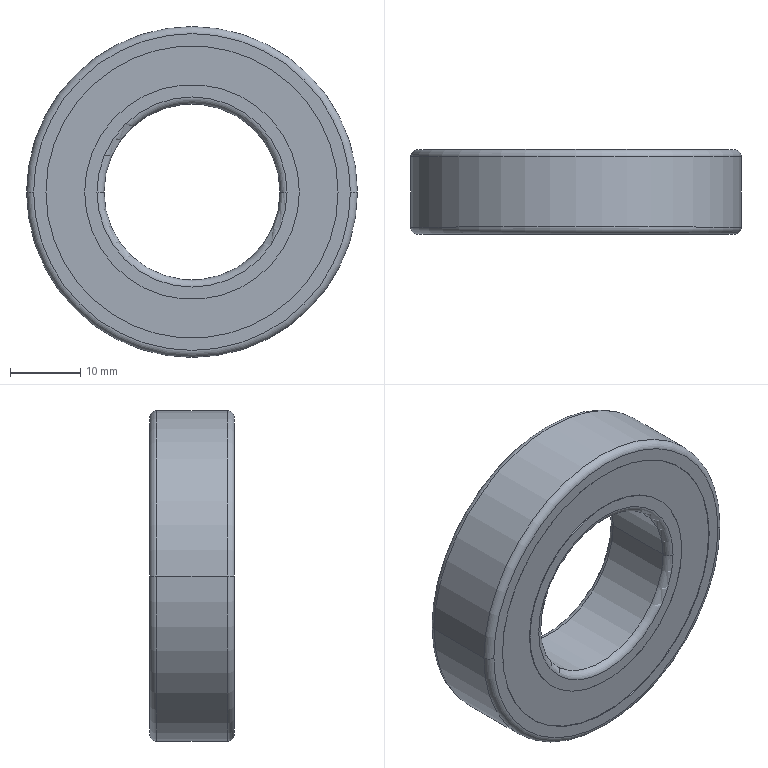Part | NX | 1 solid | 26 faces | box 47 x 12 x 47 mm | volume 14707 mm3 | cylinder 12 | torus 8 | plane 6 | commonest cylinder face diameters 30.5 x4 41.5 x4 25 x2 47 x2
STEP:
#1=CARTESIAN_POINT('',(-13.5,6.,0.));
#2=VERTEX_POINT('',#1);
#3=CARTESIAN_POINT('',(13.5,6.,0.));
#4=VERTEX_POINT('',#3);
#5=CARTESIAN_POINT('',(0.,6.,0.));
#6=DIRECTION('',(0.,1.,0.));
#7=DIRECTION('',(-1.,0.,0.));
#8=AXIS2_PLACEMENT_3D('',#5,#6,#7);
#9=CIRCLE('',#8,13.5);
#10=EDGE_CURVE('',#2,#4,#9,.T.);
#11=ORIENTED_EDGE('',*,*,#10,.T.);
#12=CARTESIAN_POINT('',(12.5,5.,0.));
#13=VERTEX_POINT('',#12);
#14=CARTESIAN_POINT('',(13.5,5.,0.));
#15=DIRECTION('',(0.,0.,1.));
#16=DIRECTION('',(1.,0.,0.));
#17=AXIS2_PLACEMENT_3D('',#14,#15,#16);
#18=CIRCLE('',#17,1.);
#19=EDGE_CURVE('',#4,#13,#18,.T.);
#20=ORIENTED_EDGE('',*,*,#19,.T.);
#21=CARTESIAN_POINT('',(-12.5,5.,0.));
#22=VERTEX_POINT('',#21);
#23=CARTESIAN_POINT('',(0.,5.,0.));
#24=DIRECTION('',(0.,-1.,0.));
#25=DIRECTION('',(-1.,0.,0.));
#26=AXIS2_PLACEMENT_3D('',#23,#24,#25);
#27=CIRCLE('',#26,12.5);
#28=EDGE_CURVE('',#13,#22,#27,.T.);
#29=ORIENTED_EDGE('',*,*,#28,.T.);
#30=CARTESIAN_POINT('',(-13.5,5.,0.));
#31=DIRECTION('',(0.,0.,-1.));
#32=DIRECTION('',(-1.,0.,0.));
#33=AXIS2_PLACEMENT_3D('',#30,#31,#32);
#34=CIRCLE('',#33,1.);
#35=EDGE_CURVE('',#2,#22,#34,.T.);
#36=ORIENTED_EDGE('',*,*,#35,.F.);
#37=EDGE_LOOP('',(#11,#20,#29,#36));
#38=FACE_BOUND('',#37,.T.);
#39=CARTESIAN_POINT('',(0.,5.,0.));
#40=DIRECTION('',(0.,-1.,0.));
#41=DIRECTION('',(-1.,0.,0.));
#42=AXIS2_PLACEMENT_3D('',#39,#40,#41);
#43=TOROIDAL_SURFACE('',#42,13.5,1.);
#44=ADVANCED_FACE('',(#38),#43,.T.);
#45=CARTESIAN_POINT('',(22.5,6.,0.));
#46=VERTEX_POINT('',#45);
#47=CARTESIAN_POINT('',(-22.5,6.,0.));
#48=VERTEX_POINT('',#47);
#49=CARTESIAN_POINT('',(0.,6.,0.));
#50=DIRECTION('',(0.,-1.,0.));
#51=DIRECTION('',(1.,0.,0.));
#52=AXIS2_PLACEMENT_3D('',#49,#50,#51);
#53=CIRCLE('',#52,22.5);
#54=EDGE_CURVE('',#46,#48,#53,.T.);
#55=ORIENTED_EDGE('',*,*,#54,.T.);
#56=CARTESIAN_POINT('',(-23.5,5.,0.));
#57=VERTEX_POINT('',#56);
#58=CARTESIAN_POINT('',(-22.5,5.,0.));
#59=DIRECTION('',(0.,0.,-1.));
#60=DIRECTION('',(-1.,0.,0.));
#61=AXIS2_PLACEMENT_3D('',#58,#59,#60);
#62=CIRCLE('',#61,1.);
#63=EDGE_CURVE('',#48,#57,#62,.F.);
#64=ORIENTED_EDGE('',*,*,#63,.T.);
#65=CARTESIAN_POINT('',(23.5,5.,0.));
#66=VERTEX_POINT('',#65);
#67=CARTESIAN_POINT('',(0.,5.,0.));
#68=DIRECTION('',(0.,-1.,0.));
#69=DIRECTION('',(-1.,0.,0.));
#70=AXIS2_PLACEMENT_3D('',#67,#68,#69);
#71=CIRCLE('',#70,23.5);
#72=EDGE_CURVE('',#66,#57,#71,.T.);
#73=ORIENTED_EDGE('',*,*,#72,.F.);
#74=CARTESIAN_POINT('',(22.5,5.,0.));
#75=DIRECTION('',(0.,0.,1.));
#76=DIRECTION('',(1.,0.,0.));
#77=AXIS2_PLACEMENT_3D('',#74,#75,#76);
#78=CIRCLE('',#77,1.);
#79=EDGE_CURVE('',#46,#66,#78,.F.);
#80=ORIENTED_EDGE('',*,*,#79,.F.);
#81=EDGE_LOOP('',(#55,#64,#73,#80));
#82=FACE_BOUND('',#81,.T.);
#83=CARTESIAN_POINT('',(0.,5.,0.));
#84=DIRECTION('',(0.,-1.,0.));
#85=DIRECTION('',(-1.,0.,0.));
#86=AXIS2_PLACEMENT_3D('',#83,#84,#85);
#87=TOROIDAL_SURFACE('',#86,22.5,1.);
#88=ADVANCED_FACE('',(#82),#87,.T.);
#89=CARTESIAN_POINT('',(0.,5.,0.));
#90=DIRECTION('',(0.,-1.,0.));
#91=DIRECTION('',(-1.,0.,0.));
#92=AXIS2_PLACEMENT_3D('',#89,#90,#91);
#93=CIRCLE('',#92,12.5);
#94=EDGE_CURVE('',#22,#13,#93,.T.);
#95=ORIENTED_EDGE('',*,*,#94,.F.);
#96=CARTESIAN_POINT('',(-12.5,-5.,0.));
#97=VERTEX_POINT('',#96);
#98=CARTESIAN_POINT('',(-12.5,6.6,0.));
#99=DIRECTION('',(0.,-1.,0.));
#100=VECTOR('',#99,1000.);
#101=LINE('',#98,#100);
#102=EDGE_CURVE('',#97,#22,#101,.F.);
#103=ORIENTED_EDGE('',*,*,#102,.F.);
#104=CARTESIAN_POINT('',(12.5,-5.,0.));
#105=VERTEX_POINT('',#104);
#106=CARTESIAN_POINT('',(0.,-5.,0.));
#107=DIRECTION('',(0.,-1.,0.));
#108=DIRECTION('',(-1.,0.,0.));
#109=AXIS2_PLACEMENT_3D('',#106,#107,#108);
#110=CIRCLE('',#109,12.5);
#111=EDGE_CURVE('',#97,#105,#110,.T.);
#112=ORIENTED_EDGE('',*,*,#111,.T.);
#113=CARTESIAN_POINT('',(12.5,6.6,0.));
#114=DIRECTION('',(0.,-1.,0.));
#115=VECTOR('',#114,1000.);
#116=LINE('',#113,#115);
#117=EDGE_CURVE('',#105,#13,#116,.F.);
#118=ORIENTED_EDGE('',*,*,#117,.T.);
#119=EDGE_LOOP('',(#95,#103,#112,#118));
#120=FACE_BOUND('',#119,.T.);
#121=CARTESIAN_POINT('',(0.,6.6,0.));
#122=DIRECTION('',(0.,-1.,0.));
#123=DIRECTION('',(-1.,0.,0.));
#124=AXIS2_PLACEMENT_3D('',#121,#122,#123);
#125=CYLINDRICAL_SURFACE('',#124,12.5);
#126=ADVANCED_FACE('',(#120),#125,.F.);
#127=CARTESIAN_POINT('',(-20.75,5.9,0.));
#128=VERTEX_POINT('',#127);
#129=CARTESIAN_POINT('',(20.75,5.9,0.));
#130=VERTEX_POINT('',#129);
#131=CARTESIAN_POINT('',(0.,5.9,0.));
#132=DIRECTION('',(0.,-1.,0.));
#133=DIRECTION('',(1.,0.,0.));
#134=AXIS2_PLACEMENT_3D('',#131,#132,#133);
#135=CIRCLE('',#134,20.75);
#136=EDGE_CURVE('',#128,#130,#135,.T.);
#137=ORIENTED_EDGE('',*,*,#136,.T.);
#138=CARTESIAN_POINT('',(20.75,6.,0.));
#139=VERTEX_POINT('',#138);
#140=CARTESIAN_POINT('',(20.75,6.6,0.));
#141=DIRECTION('',(0.,-1.,0.));
#142=VECTOR('',#141,1000.);
#143=LINE('',#140,#142);
#144=EDGE_CURVE('',#139,#130,#143,.T.);
#145=ORIENTED_EDGE('',*,*,#144,.F.);
#146=CARTESIAN_POINT('',(-20.75,6.,0.));
#147=VERTEX_POINT('',#146);
#148=CARTESIAN_POINT('',(0.,6.,0.));
#149=DIRECTION('',(0.,1.,0.));
#150=DIRECTION('',(1.,0.,0.));
#151=AXIS2_PLACEMENT_3D('',#148,#149,#150);
#152=CIRCLE('',#151,20.75);
#153=EDGE_CURVE('',#139,#147,#152,.T.);
#154=ORIENTED_EDGE('',*,*,#153,.T.);
#155=CARTESIAN_POINT('',(-20.75,6.6,0.));
#156=DIRECTION('',(0.,-1.,0.));
#157=VECTOR('',#156,1000.);
#158=LINE('',#155,#157);
#159=EDGE_CURVE('',#147,#128,#158,.T.);
#160=ORIENTED_EDGE('',*,*,#159,.T.);
#161=EDGE_LOOP('',(#137,#145,#154,#160));
#162=FACE_BOUND('',#161,.T.);
#163=CARTESIAN_POINT('',(0.,6.6,0.));
#164=DIRECTION('',(0.,-1.,0.));
#165=DIRECTION('',(-1.,0.,0.));
#166=AXIS2_PLACEMENT_3D('',#163,#164,#165);
#167=CYLINDRICAL_SURFACE('',#166,20.75);
#168=ADVANCED_FACE('',(#162),#167,.F.);
#169=ORIENTED_EDGE('',*,*,#111,.F.);
#170=CARTESIAN_POINT('',(-13.5,-6.,0.));
#171=VERTEX_POINT('',#170);
#172=CARTESIAN_POINT('',(-13.5,-5.,0.));
#173=DIRECTION('',(0.,0.,-1.));
#174=DIRECTION('',(-1.,0.,0.));
#175=AXIS2_PLACEMENT_3D('',#172,#173,#174);
#176=CIRCLE('',#175,1.);
#177=EDGE_CURVE('',#171,#97,#176,.F.);
#178=ORIENTED_EDGE('',*,*,#177,.F.);
#179=CARTESIAN_POINT('',(13.5,-6.,0.));
#180=VERTEX_POINT('',#179);
#181=CARTESIAN_POINT('',(0.,-6.,0.));
#182=DIRECTION('',(0.,-1.,0.));
#183=DIRECTION('',(1.,0.,0.));
#184=AXIS2_PLACEMENT_3D('',#181,#182,#183);
#185=CIRCLE('',#184,13.5);
#186=EDGE_CURVE('',#171,#180,#185,.T.);
#187=ORIENTED_EDGE('',*,*,#186,.T.);
#188=CARTESIAN_POINT('',(13.5,-5.,0.));
#189=DIRECTION('',(0.,0.,1.));
#190=DIRECTION('',(1.,0.,0.));
#191=AXIS2_PLACEMENT_3D('',#188,#189,#190);
#192=CIRCLE('',#191,1.);
#193=EDGE_CURVE('',#180,#105,#192,.F.);
#194=ORIENTED_EDGE('',*,*,#193,.T.);
#195=EDGE_LOOP('',(#169,#178,#187,#194));
#196=FACE_BOUND('',#195,.T.);
#197=CARTESIAN_POINT('',(0.,-5.,0.));
#198=DIRECTION('',(0.,-1.,0.));
#199=DIRECTION('',(-1.,0.,0.));
#200=AXIS2_PLACEMENT_3D('',#197,#198,#199);
#201=TOROIDAL_SURFACE('',#200,13.5,1.);
#202=ADVANCED_FACE('',(#196),#201,.T.);
#203=ORIENTED_EDGE('',*,*,#54,.F.);
#204=CARTESIAN_POINT('',(0.,6.,0.));
#205=DIRECTION('',(0.,-1.,0.));
#206=DIRECTION('',(1.,0.,0.));
#207=AXIS2_PLACEMENT_3D('',#204,#205,#206);
#208=CIRCLE('',#207,22.5);
#209=EDGE_CURVE('',#48,#46,#208,.T.);
#210=ORIENTED_EDGE('',*,*,#209,.F.);
#211=EDGE_LOOP('',(#203,#210));
#212=FACE_BOUND('',#211,.T.);
#213=CARTESIAN_POINT('',(0.,6.,0.));
#214=DIRECTION('',(0.,1.,0.));
#215=DIRECTION('',(1.,0.,0.));
#216=AXIS2_PLACEMENT_3D('',#213,#214,#215);
#217=CIRCLE('',#216,20.75);
#218=EDGE_CURVE('',#147,#139,#217,.T.);
#219=ORIENTED_EDGE('',*,*,#218,.F.);
#220=ORIENTED_EDGE('',*,*,#153,.F.);
#221=EDGE_LOOP('',(#219,#220));
#222=FACE_BOUND('',#221,.T.);
#223=CARTESIAN_POINT('',(0.,6.,0.));
#224=DIRECTION('',(0.,-1.,0.));
#225=DIRECTION('',(0.,0.,-1.));
#226=AXIS2_PLACEMENT_3D('',#223,#224,#225);
#227=PLANE('',#226);
#228=ADVANCED_FACE('',(#212,#222),#227,.F.);
#229=CARTESIAN_POINT('',(15.25,-6.,0.));
#230=VERTEX_POINT('',#229);
#231=CARTESIAN_POINT('',(-15.25,-6.,0.));
#232=VERTEX_POINT('',#231);
#233=CARTESIAN_POINT('',(0.,-6.,0.));
#234=DIRECTION('',(0.,1.,0.));
#235=DIRECTION('',(1.,0.,0.));
#236=AXIS2_PLACEMENT_3D('',#233,#234,#235);
#237=CIRCLE('',#236,15.25);
#238=EDGE_CURVE('',#230,#232,#237,.T.);
#239=ORIENTED_EDGE('',*,*,#238,.F.);
#240=CARTESIAN_POINT('',(0.,-6.,0.));
#241=DIRECTION('',(0.,1.,0.));
#242=DIRECTION('',(1.,0.,0.));
#243=AXIS2_PLACEMENT_3D('',#240,#241,#242);
#244=CIRCLE('',#243,15.25);
#245=EDGE_CURVE('',#232,#230,#244,.T.);
#246=ORIENTED_EDGE('',*,*,#245,.F.);
#247=EDGE_LOOP('',(#239,#246));
#248=FACE_BOUND('',#247,.T.);
#249=CARTESIAN_POINT('',(0.,-6.,0.));
#250=DIRECTION('',(0.,-1.,0.));
#251=DIRECTION('',(1.,0.,0.));
#252=AXIS2_PLACEMENT_3D('',#249,#250,#251);
#253=CIRCLE('',#252,13.5);
#254=EDGE_CURVE('',#180,#171,#253,.T.);
#255=ORIENTED_EDGE('',*,*,#254,.F.);
#256=ORIENTED_EDGE('',*,*,#186,.F.);
#257=EDGE_LOOP('',(#255,#256));
#258=FACE_BOUND('',#257,.T.);
#259=CARTESIAN_POINT('',(0.,-6.,0.));
#260=DIRECTION('',(0.,-1.,0.));
#261=DIRECTION('',(0.,0.,-1.));
#262=AXIS2_PLACEMENT_3D('',#259,#260,#261);
#263=PLANE('',#262);
#264=ADVANCED_FACE('',(#248,#258),#263,.T.);
#265=ORIENTED_EDGE('',*,*,#238,.T.);
#266=CARTESIAN_POINT('',(-15.25,-5.9,0.));
#267=VERTEX_POINT('',#266);
#268=CARTESIAN_POINT('',(-15.25,6.6,0.));
#269=DIRECTION('',(0.,-1.,0.));
#270=VECTOR('',#269,1000.);
#271=LINE('',#268,#270);
#272=EDGE_CURVE('',#232,#267,#271,.F.);
#273=ORIENTED_EDGE('',*,*,#272,.T.);
#274=CARTESIAN_POINT('',(15.25,-5.9,0.));
#275=VERTEX_POINT('',#274);
#276=CARTESIAN_POINT('',(0.,-5.9,0.));
#277=DIRECTION('',(0.,-1.,0.));
#278=DIRECTION('',(1.,0.,0.));
#279=AXIS2_PLACEMENT_3D('',#276,#277,#278);
#280=CIRCLE('',#279,15.25);
#281=EDGE_CURVE('',#267,#275,#280,.T.);
#282=ORIENTED_EDGE('',*,*,#281,.T.);
#283=CARTESIAN_POINT('',(15.25,6.6,0.));
#284=DIRECTION('',(0.,-1.,0.));
#285=VECTOR('',#284,1000.);
#286=LINE('',#283,#285);
#287=EDGE_CURVE('',#230,#275,#286,.F.);
#288=ORIENTED_EDGE('',*,*,#287,.F.);
#289=EDGE_LOOP('',(#265,#273,#282,#288));
#290=FACE_BOUND('',#289,.T.);
#291=CARTESIAN_POINT('',(0.,6.6,0.));
#292=DIRECTION('',(0.,-1.,0.));
#293=DIRECTION('',(-1.,0.,0.));
#294=AXIS2_PLACEMENT_3D('',#291,#292,#293);
#295=CYLINDRICAL_SURFACE('',#294,15.25);
#296=ADVANCED_FACE('',(#290),#295,.T.);
#297=CARTESIAN_POINT('',(15.25,6.,0.));
#298=VERTEX_POINT('',#297);
#299=CARTESIAN_POINT('',(-15.25,6.,0.));
#300=VERTEX_POINT('',#299);
#301=CARTESIAN_POINT('',(0.,6.,0.));
#302=DIRECTION('',(0.,-1.,0.));
#303=DIRECTION('',(1.,0.,0.));
#304=AXIS2_PLACEMENT_3D('',#301,#302,#303);
#305=CIRCLE('',#304,15.25);
#306=EDGE_CURVE('',#298,#300,#305,.T.);
#307=ORIENTED_EDGE('',*,*,#306,.F.);
#308=CARTESIAN_POINT('',(0.,6.,0.));
#309=DIRECTION('',(0.,-1.,0.));
#310=DIRECTION('',(1.,0.,0.));
#311=AXIS2_PLACEMENT_3D('',#308,#309,#310);
#312=CIRCLE('',#311,15.25);
#313=EDGE_CURVE('',#300,#298,#312,.T.);
#314=ORIENTED_EDGE('',*,*,#313,.F.);
#315=EDGE_LOOP('',(#307,#314));
#316=FACE_BOUND('',#315,.T.);
#317=ORIENTED_EDGE('',*,*,#10,.F.);
#318=CARTESIAN_POINT('',(0.,6.,0.));
#319=DIRECTION('',(0.,1.,0.));
#320=DIRECTION('',(-1.,0.,0.));
#321=AXIS2_PLACEMENT_3D('',#318,#319,#320);
#322=CIRCLE('',#321,13.5);
#323=EDGE_CURVE('',#4,#2,#322,.T.);
#324=ORIENTED_EDGE('',*,*,#323,.F.);
#325=EDGE_LOOP('',(#317,#324));
#326=FACE_BOUND('',#325,.T.);
#327=CARTESIAN_POINT('',(0.,6.,0.));
#328=DIRECTION('',(0.,-1.,0.));
#329=DIRECTION('',(0.,0.,-1.));
#330=AXIS2_PLACEMENT_3D('',#327,#328,#329);
#331=PLANE('',#330);
#332=ADVANCED_FACE('',(#316,#326),#331,.F.);
#333=CARTESIAN_POINT('',(20.75,-5.9,0.));
#334=VERTEX_POINT('',#333);
#335=CARTESIAN_POINT('',(-20.75,-5.9,0.));
#336=VERTEX_POINT('',#335);
#337=CARTESIAN_POINT('',(0.,-5.9,0.));
#338=DIRECTION('',(0.,1.,0.));
#339=DIRECTION('',(1.,0.,0.));
#340=AXIS2_PLACEMENT_3D('',#337,#338,#339);
#341=CIRCLE('',#340,20.75);
#342=EDGE_CURVE('',#334,#336,#341,.T.);
#343=ORIENTED_EDGE('',*,*,#342,.F.);
#344=CARTESIAN_POINT('',(0.,-5.9,0.));
#345=DIRECTION('',(0.,1.,0.));
#346=DIRECTION('',(1.,0.,0.));
#347=AXIS2_PLACEMENT_3D('',#344,#345,#346);
#348=CIRCLE('',#347,20.75);
#349=EDGE_CURVE('',#336,#334,#348,.T.);
#350=ORIENTED_EDGE('',*,*,#349,.F.);
#351=EDGE_LOOP('',(#343,#350));
#352=FACE_BOUND('',#351,.T.);
#353=CARTESIAN_POINT('',(0.,-5.9,0.));
#354=DIRECTION('',(0.,-1.,0.));
#355=DIRECTION('',(1.,0.,0.));
#356=AXIS2_PLACEMENT_3D('',#353,#354,#355);
#357=CIRCLE('',#356,15.25);
#358=EDGE_CURVE('',#275,#267,#357,.T.);
#359=ORIENTED_EDGE('',*,*,#358,.F.);
#360=ORIENTED_EDGE('',*,*,#281,.F.);
#361=EDGE_LOOP('',(#359,#360));
#362=FACE_BOUND('',#361,.T.);
#363=CARTESIAN_POINT('',(0.,-5.9,0.));
#364=DIRECTION('',(0.,-1.,0.));
#365=DIRECTION('',(0.,0.,-1.));
#366=AXIS2_PLACEMENT_3D('',#363,#364,#365);
#367=PLANE('',#366);
#368=ADVANCED_FACE('',(#352,#362),#367,.T.);
#369=ORIENTED_EDGE('',*,*,#342,.T.);
#370=CARTESIAN_POINT('',(-20.75,-6.,0.));
#371=VERTEX_POINT('',#370);
#372=CARTESIAN_POINT('',(-20.75,6.6,0.));
#373=DIRECTION('',(0.,-1.,0.));
#374=VECTOR('',#373,1000.);
#375=LINE('',#372,#374);
#376=EDGE_CURVE('',#371,#336,#375,.F.);
#377=ORIENTED_EDGE('',*,*,#376,.F.);
#378=CARTESIAN_POINT('',(20.75,-6.,0.));
#379=VERTEX_POINT('',#378);
#380=CARTESIAN_POINT('',(0.,-6.,0.));
#381=DIRECTION('',(0.,-1.,0.));
#382=DIRECTION('',(1.,0.,0.));
#383=AXIS2_PLACEMENT_3D('',#380,#381,#382);
#384=CIRCLE('',#383,20.75);
#385=EDGE_CURVE('',#371,#379,#384,.T.);
#386=ORIENTED_EDGE('',*,*,#385,.T.);
#387=CARTESIAN_POINT('',(20.75,6.6,0.));
#388=DIRECTION('',(0.,-1.,0.));
#389=VECTOR('',#388,1000.);
#390=LINE('',#387,#389);
#391=EDGE_CURVE('',#379,#334,#390,.F.);
#392=ORIENTED_EDGE('',*,*,#391,.T.);
#393=EDGE_LOOP('',(#369,#377,#386,#392));
#394=FACE_BOUND('',#393,.T.);
#395=CARTESIAN_POINT('',(0.,6.6,0.));
#396=DIRECTION('',(0.,-1.,0.));
#397=DIRECTION('',(-1.,0.,0.));
#398=AXIS2_PLACEMENT_3D('',#395,#396,#397);
#399=CYLINDRICAL_SURFACE('',#398,20.75);
#400=ADVANCED_FACE('',(#394),#399,.F.);
#401=CARTESIAN_POINT('',(15.25,5.9,0.));
#402=VERTEX_POINT('',#401);
#403=CARTESIAN_POINT('',(-15.25,5.9,0.));
#404=VERTEX_POINT('',#403);
#405=CARTESIAN_POINT('',(0.,5.9,0.));
#406=DIRECTION('',(0.,1.,0.));
#407=DIRECTION('',(1.,0.,0.));
#408=AXIS2_PLACEMENT_3D('',#405,#406,#407);
#409=CIRCLE('',#408,15.25);
#410=EDGE_CURVE('',#402,#404,#409,.T.);
#411=ORIENTED_EDGE('',*,*,#410,.T.);
#412=CARTESIAN_POINT('',(-15.25,6.6,0.));
#413=DIRECTION('',(0.,-1.,0.));
#414=VECTOR('',#413,1000.);
#415=LINE('',#412,#414);
#416=EDGE_CURVE('',#404,#300,#415,.F.);
#417=ORIENTED_EDGE('',*,*,#416,.T.);
#418=ORIENTED_EDGE('',*,*,#313,.T.);
#419=CARTESIAN_POINT('',(15.25,6.6,0.));
#420=DIRECTION('',(0.,-1.,0.));
#421=VECTOR('',#420,1000.);
#422=LINE('',#419,#421);
#423=EDGE_CURVE('',#402,#298,#422,.F.);
#424=ORIENTED_EDGE('',*,*,#423,.F.);
#425=EDGE_LOOP('',(#411,#417,#418,#424));
#426=FACE_BOUND('',#425,.T.);
#427=CARTESIAN_POINT('',(0.,6.6,0.));
#428=DIRECTION('',(0.,-1.,0.));
#429=DIRECTION('',(-1.,0.,0.));
#430=AXIS2_PLACEMENT_3D('',#427,#428,#429);
#431=CYLINDRICAL_SURFACE('',#430,15.25);
#432=ADVANCED_FACE('',(#426),#431,.T.);
#433=CARTESIAN_POINT('',(22.5,-6.,0.));
#434=VERTEX_POINT('',#433);
#435=CARTESIAN_POINT('',(-22.5,-6.,0.));
#436=VERTEX_POINT('',#435);
#437=CARTESIAN_POINT('',(0.,-6.,0.));
#438=DIRECTION('',(0.,1.,0.));
#439=DIRECTION('',(1.,0.,0.));
#440=AXIS2_PLACEMENT_3D('',#437,#438,#439);
#441=CIRCLE('',#440,22.5);
#442=EDGE_CURVE('',#434,#436,#441,.T.);
#443=ORIENTED_EDGE('',*,*,#442,.F.);
#444=CARTESIAN_POINT('',(0.,-6.,0.));
#445=DIRECTION('',(0.,1.,0.));
#446=DIRECTION('',(1.,0.,0.));
#447=AXIS2_PLACEMENT_3D('',#444,#445,#446);
#448=CIRCLE('',#447,22.5);
#449=EDGE_CURVE('',#436,#434,#448,.T.);
#450=ORIENTED_EDGE('',*,*,#449,.F.);
#451=EDGE_LOOP('',(#443,#450));
#452=FACE_BOUND('',#451,.T.);
#453=ORIENTED_EDGE('',*,*,#385,.F.);
#454=CARTESIAN_POINT('',(0.,-6.,0.));
#455=DIRECTION('',(0.,-1.,0.));
#456=DIRECTION('',(1.,0.,0.));
#457=AXIS2_PLACEMENT_3D('',#454,#455,#456);
#458=CIRCLE('',#457,20.75);
#459=EDGE_CURVE('',#379,#371,#458,.T.);
#460=ORIENTED_EDGE('',*,*,#459,.F.);
#461=EDGE_LOOP('',(#453,#460));
#462=FACE_BOUND('',#461,.T.);
#463=CARTESIAN_POINT('',(0.,-6.,0.));
#464=DIRECTION('',(0.,-1.,0.));
#465=DIRECTION('',(0.,0.,-1.));
#466=AXIS2_PLACEMENT_3D('',#463,#464,#465);
#467=PLANE('',#466);
#468=ADVANCED_FACE('',(#452,#462),#467,.T.);
#469=ORIENTED_EDGE('',*,*,#442,.T.);
#470=CARTESIAN_POINT('',(-23.5,-5.,0.));
#471=VERTEX_POINT('',#470);
#472=CARTESIAN_POINT('',(-22.5,-5.,0.));
#473=DIRECTION('',(0.,0.,-1.));
#474=DIRECTION('',(-1.,0.,0.));
#475=AXIS2_PLACEMENT_3D('',#472,#473,#474);
#476=CIRCLE('',#475,1.);
#477=EDGE_CURVE('',#471,#436,#476,.F.);
#478=ORIENTED_EDGE('',*,*,#477,.F.);
#479=CARTESIAN_POINT('',(23.5,-5.,0.));
#480=VERTEX_POINT('',#479);
#481=CARTESIAN_POINT('',(0.,-5.,0.));
#482=DIRECTION('',(0.,-1.,0.));
#483=DIRECTION('',(-1.,0.,0.));
#484=AXIS2_PLACEMENT_3D('',#481,#482,#483);
#485=CIRCLE('',#484,23.5);
#486=EDGE_CURVE('',#471,#480,#485,.T.);
#487=ORIENTED_EDGE('',*,*,#486,.T.);
#488=CARTESIAN_POINT('',(22.5,-5.,0.));
#489=DIRECTION('',(0.,0.,1.));
#490=DIRECTION('',(1.,0.,0.));
#491=AXIS2_PLACEMENT_3D('',#488,#489,#490);
#492=CIRCLE('',#491,1.);
#493=EDGE_CURVE('',#480,#434,#492,.F.);
#494=ORIENTED_EDGE('',*,*,#493,.T.);
#495=EDGE_LOOP('',(#469,#478,#487,#494));
#496=FACE_BOUND('',#495,.T.);
#497=CARTESIAN_POINT('',(0.,-5.,0.));
#498=DIRECTION('',(0.,-1.,0.));
#499=DIRECTION('',(-1.,0.,0.));
#500=AXIS2_PLACEMENT_3D('',#497,#498,#499);
#501=TOROIDAL_SURFACE('',#500,22.5,1.);
#502=ADVANCED_FACE('',(#496),#501,.T.);
#503=ORIENTED_EDGE('',*,*,#136,.F.);
#504=CARTESIAN_POINT('',(0.,5.9,0.));
#505=DIRECTION('',(0.,-1.,0.));
#506=DIRECTION('',(1.,0.,0.));
#507=AXIS2_PLACEMENT_3D('',#504,#505,#506);
#508=CIRCLE('',#507,20.75);
#509=EDGE_CURVE('',#130,#128,#508,.T.);
#510=ORIENTED_EDGE('',*,*,#509,.F.);
#511=EDGE_LOOP('',(#503,#510));
#512=FACE_BOUND('',#511,.T.);
#513=ORIENTED_EDGE('',*,*,#410,.F.);
#514=CARTESIAN_POINT('',(0.,5.9,0.));
#515=DIRECTION('',(0.,1.,0.));
#516=DIRECTION('',(1.,0.,0.));
#517=AXIS2_PLACEMENT_3D('',#514,#515,#516);
#518=CIRCLE('',#517,15.25);
#519=EDGE_CURVE('',#404,#402,#518,.T.);
#520=ORIENTED_EDGE('',*,*,#519,.F.);
#521=EDGE_LOOP('',(#513,#520));
#522=FACE_BOUND('',#521,.T.);
#523=CARTESIAN_POINT('',(0.,5.9,0.));
#524=DIRECTION('',(0.,-1.,0.));
#525=DIRECTION('',(0.,0.,-1.));
#526=AXIS2_PLACEMENT_3D('',#523,#524,#525);
#527=PLANE('',#526);
#528=ADVANCED_FACE('',(#512,#522),#527,.F.);
#529=CARTESIAN_POINT('',(0.,-5.,0.));
#530=DIRECTION('',(0.,-1.,0.));
#531=DIRECTION('',(-1.,0.,0.));
#532=AXIS2_PLACEMENT_3D('',#529,#530,#531);
#533=CIRCLE('',#532,23.5);
#534=EDGE_CURVE('',#480,#471,#533,.T.);
#535=ORIENTED_EDGE('',*,*,#534,.F.);
#536=CARTESIAN_POINT('',(23.5,6.6,0.));
#537=DIRECTION('',(0.,-1.,0.));
#538=VECTOR('',#537,1000.);
#539=LINE('',#536,#538);
#540=EDGE_CURVE('',#480,#66,#539,.F.);
#541=ORIENTED_EDGE('',*,*,#540,.T.);
#542=ORIENTED_EDGE('',*,*,#72,.T.);
#543=CARTESIAN_POINT('',(-23.5,6.6,0.));
#544=DIRECTION('',(0.,-1.,0.));
#545=VECTOR('',#544,1000.);
#546=LINE('',#543,#545);
#547=EDGE_CURVE('',#471,#57,#546,.F.);
#548=ORIENTED_EDGE('',*,*,#547,.F.);
#549=EDGE_LOOP('',(#535,#541,#542,#548));
#550=FACE_BOUND('',#549,.T.);
#551=CARTESIAN_POINT('',(0.,6.6,0.));
#552=DIRECTION('',(0.,-1.,0.));
#553=DIRECTION('',(-1.,0.,0.));
#554=AXIS2_PLACEMENT_3D('',#551,#552,#553);
#555=CYLINDRICAL_SURFACE('',#554,23.5);
#556=ADVANCED_FACE('',(#550),#555,.T.);
#557=ORIENTED_EDGE('',*,*,#306,.T.);
#558=ORIENTED_EDGE('',*,*,#416,.F.);
#559=ORIENTED_EDGE('',*,*,#519,.T.);
#560=ORIENTED_EDGE('',*,*,#423,.T.);
#561=EDGE_LOOP('',(#557,#558,#559,#560));
#562=FACE_BOUND('',#561,.T.);
#563=CARTESIAN_POINT('',(0.,6.6,0.));
#564=DIRECTION('',(0.,-1.,0.));
#565=DIRECTION('',(-1.,0.,0.));
#566=AXIS2_PLACEMENT_3D('',#563,#564,#565);
#567=CYLINDRICAL_SURFACE('',#566,15.25);
#568=ADVANCED_FACE('',(#562),#567,.T.);
#569=ORIENTED_EDGE('',*,*,#102,.T.);
#570=ORIENTED_EDGE('',*,*,#28,.F.);
#571=ORIENTED_EDGE('',*,*,#117,.F.);
#572=CARTESIAN_POINT('',(0.,-5.,0.));
#573=DIRECTION('',(0.,-1.,0.));
#574=DIRECTION('',(-1.,0.,0.));
#575=AXIS2_PLACEMENT_3D('',#572,#573,#574);
#576=CIRCLE('',#575,12.5);
#577=EDGE_CURVE('',#105,#97,#576,.T.);
#578=ORIENTED_EDGE('',*,*,#577,.T.);
#579=EDGE_LOOP('',(#569,#570,#571,#578));
#580=FACE_BOUND('',#579,.T.);
#581=CARTESIAN_POINT('',(0.,6.6,0.));
#582=DIRECTION('',(0.,-1.,0.));
#583=DIRECTION('',(-1.,0.,0.));
#584=AXIS2_PLACEMENT_3D('',#581,#582,#583);
#585=CYLINDRICAL_SURFACE('',#584,12.5);
#586=ADVANCED_FACE('',(#580),#585,.F.);
#587=ORIENTED_EDGE('',*,*,#358,.T.);
#588=ORIENTED_EDGE('',*,*,#272,.F.);
#589=ORIENTED_EDGE('',*,*,#245,.T.);
#590=ORIENTED_EDGE('',*,*,#287,.T.);
#591=EDGE_LOOP('',(#587,#588,#589,#590));
#592=FACE_BOUND('',#591,.T.);
#593=CARTESIAN_POINT('',(0.,6.6,0.));
#594=DIRECTION('',(0.,-1.,0.));
#595=DIRECTION('',(-1.,0.,0.));
#596=AXIS2_PLACEMENT_3D('',#593,#594,#595);
#597=CYLINDRICAL_SURFACE('',#596,15.25);
#598=ADVANCED_FACE('',(#592),#597,.T.);
#599=ORIENTED_EDGE('',*,*,#376,.T.);
#600=ORIENTED_EDGE('',*,*,#349,.T.);
#601=ORIENTED_EDGE('',*,*,#391,.F.);
#602=ORIENTED_EDGE('',*,*,#459,.T.);
#603=EDGE_LOOP('',(#599,#600,#601,#602));
#604=FACE_BOUND('',#603,.T.);
#605=CARTESIAN_POINT('',(0.,6.6,0.));
#606=DIRECTION('',(0.,-1.,0.));
#607=DIRECTION('',(-1.,0.,0.));
#608=AXIS2_PLACEMENT_3D('',#605,#606,#607);
#609=CYLINDRICAL_SURFACE('',#608,20.75);
#610=ADVANCED_FACE('',(#604),#609,.F.);
#611=ORIENTED_EDGE('',*,*,#547,.T.);
#612=CARTESIAN_POINT('',(0.,5.,0.));
#613=DIRECTION('',(0.,-1.,0.));
#614=DIRECTION('',(-1.,0.,0.));
#615=AXIS2_PLACEMENT_3D('',#612,#613,#614);
#616=CIRCLE('',#615,23.5);
#617=EDGE_CURVE('',#57,#66,#616,.T.);
#618=ORIENTED_EDGE('',*,*,#617,.T.);
#619=ORIENTED_EDGE('',*,*,#540,.F.);
#620=ORIENTED_EDGE('',*,*,#486,.F.);
#621=EDGE_LOOP('',(#611,#618,#619,#620));
#622=FACE_BOUND('',#621,.T.);
#623=CARTESIAN_POINT('',(0.,6.6,0.));
#624=DIRECTION('',(0.,-1.,0.));
#625=DIRECTION('',(-1.,0.,0.));
#626=AXIS2_PLACEMENT_3D('',#623,#624,#625);
#627=CYLINDRICAL_SURFACE('',#626,23.5);
#628=ADVANCED_FACE('',(#622),#627,.T.);
#629=ORIENTED_EDGE('',*,*,#218,.T.);
#630=ORIENTED_EDGE('',*,*,#144,.T.);
#631=ORIENTED_EDGE('',*,*,#509,.T.);
#632=ORIENTED_EDGE('',*,*,#159,.F.);
#633=EDGE_LOOP('',(#629,#630,#631,#632));
#634=FACE_BOUND('',#633,.T.);
#635=CARTESIAN_POINT('',(0.,6.6,0.));
#636=DIRECTION('',(0.,-1.,0.));
#637=DIRECTION('',(-1.,0.,0.));
#638=AXIS2_PLACEMENT_3D('',#635,#636,#637);
#639=CYLINDRICAL_SURFACE('',#638,20.75);
#640=ADVANCED_FACE('',(#634),#639,.F.);
#641=ORIENTED_EDGE('',*,*,#254,.T.);
#642=ORIENTED_EDGE('',*,*,#177,.T.);
#643=ORIENTED_EDGE('',*,*,#577,.F.);
#644=ORIENTED_EDGE('',*,*,#193,.F.);
#645=EDGE_LOOP('',(#641,#642,#643,#644));
#646=FACE_BOUND('',#645,.T.);
#647=CARTESIAN_POINT('',(0.,-5.,0.));
#648=DIRECTION('',(0.,-1.,0.));
#649=DIRECTION('',(-1.,0.,0.));
#650=AXIS2_PLACEMENT_3D('',#647,#648,#649);
#651=TOROIDAL_SURFACE('',#650,13.5,1.);
#652=ADVANCED_FACE('',(#646),#651,.T.);
#653=ORIENTED_EDGE('',*,*,#534,.T.);
#654=ORIENTED_EDGE('',*,*,#477,.T.);
#655=ORIENTED_EDGE('',*,*,#449,.T.);
#656=ORIENTED_EDGE('',*,*,#493,.F.);
#657=EDGE_LOOP('',(#653,#654,#655,#656));
#658=FACE_BOUND('',#657,.T.);
#659=CARTESIAN_POINT('',(0.,-5.,0.));
#660=DIRECTION('',(0.,-1.,0.));
#661=DIRECTION('',(-1.,0.,0.));
#662=AXIS2_PLACEMENT_3D('',#659,#660,#661);
#663=TOROIDAL_SURFACE('',#662,22.5,1.);
#664=ADVANCED_FACE('',(#658),#663,.T.);
#665=ORIENTED_EDGE('',*,*,#63,.F.);
#666=ORIENTED_EDGE('',*,*,#209,.T.);
#667=ORIENTED_EDGE('',*,*,#79,.T.);
#668=ORIENTED_EDGE('',*,*,#617,.F.);
#669=EDGE_LOOP('',(#665,#666,#667,#668));
#670=FACE_BOUND('',#669,.T.);
#671=CARTESIAN_POINT('',(0.,5.,0.));
#672=DIRECTION('',(0.,-1.,0.));
#673=DIRECTION('',(-1.,0.,0.));
#674=AXIS2_PLACEMENT_3D('',#671,#672,#673);
#675=TOROIDAL_SURFACE('',#674,22.5,1.);
#676=ADVANCED_FACE('',(#670),#675,.T.);
#677=ORIENTED_EDGE('',*,*,#94,.T.);
#678=ORIENTED_EDGE('',*,*,#19,.F.);
#679=ORIENTED_EDGE('',*,*,#323,.T.);
#680=ORIENTED_EDGE('',*,*,#35,.T.);
#681=EDGE_LOOP('',(#677,#678,#679,#680));
#682=FACE_BOUND('',#681,.T.);
#683=CARTESIAN_POINT('',(0.,5.,0.));
#684=DIRECTION('',(0.,-1.,0.));
#685=DIRECTION('',(-1.,0.,0.));
#686=AXIS2_PLACEMENT_3D('',#683,#684,#685);
#687=TOROIDAL_SURFACE('',#686,13.5,1.);
#688=ADVANCED_FACE('',(#682),#687,.T.);
#689=CLOSED_SHELL('',(#44,#88,#126,#168,#202,#228,#264,#296,#332,#368,#400,#432,#468,#502,#528,#556,#568,#586,#598,#610,#628,#640,#652,#664,#676,#688));
#690=MANIFOLD_SOLID_BREP('',#689);
#691=(LENGTH_UNIT()NAMED_UNIT(*)SI_UNIT(.MILLI.,.METRE.));
#692=UNCERTAINTY_MEASURE_WITH_UNIT(LENGTH_MEASURE(0.00001),#691,'','');
#693=(NAMED_UNIT(*)PLANE_ANGLE_UNIT()SI_UNIT($,.RADIAN.));
#694=(NAMED_UNIT(*)SI_UNIT($,.STERADIAN.)SOLID_ANGLE_UNIT());
#695=(GEOMETRIC_REPRESENTATION_CONTEXT(3)GLOBAL_UNCERTAINTY_ASSIGNED_CONTEXT((#692))GLOBAL_UNIT_ASSIGNED_CONTEXT((#691,#693,#694))REPRESENTATION_CONTEXT('',''));
#696=ADVANCED_BREP_SHAPE_REPRESENTATION('',(#690),#695);